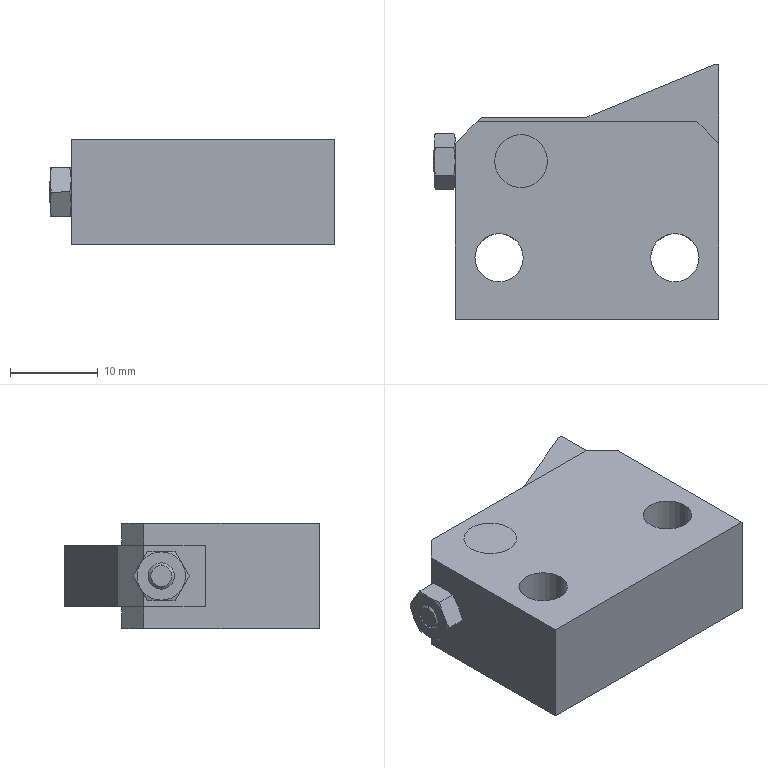Part | STEP file | Check valve assembly ATBJ7SA-S-BL | 4 solids | 91 faces | box 32.5 x 29 x 12 mm | volume 7437 mm3 | plane 41 | cylinder 26 | cone 24 | commonest cylinder face diameters 6 x8 3 x4 5 x4 5.5 x4 2.459 x2 3.04 x2